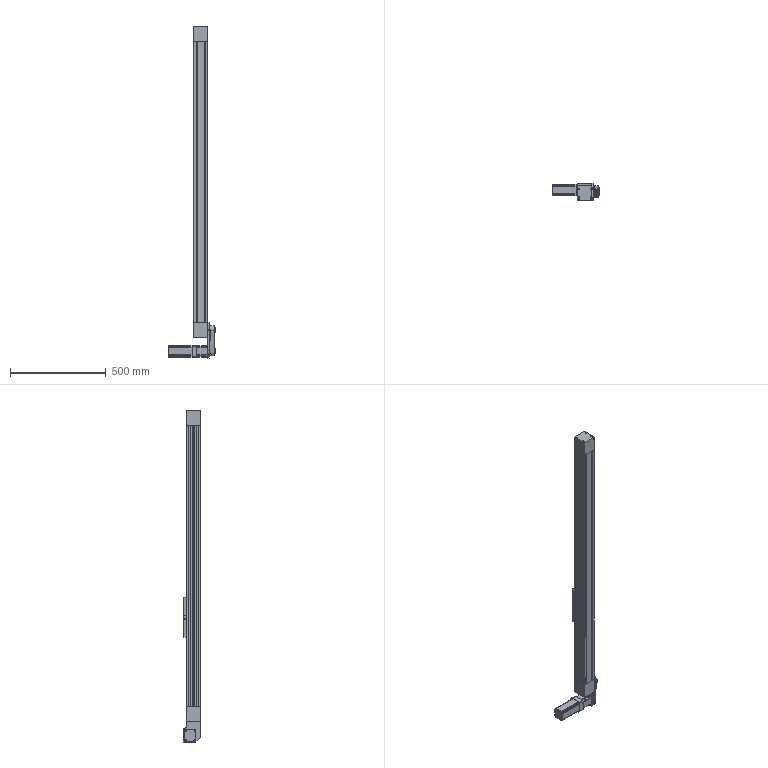Part | SolidWorks | 14 solids | 780 faces | box 249.5 x 90 x 1730 mm | volume 9701440 mm3 | plane 382 | cylinder 322 | cone 64 | torus 12 | commonest cylinder face diameters 38.65 x52 5 x39 4 x26 3.3 x22 4.2 x18 6.8 x18